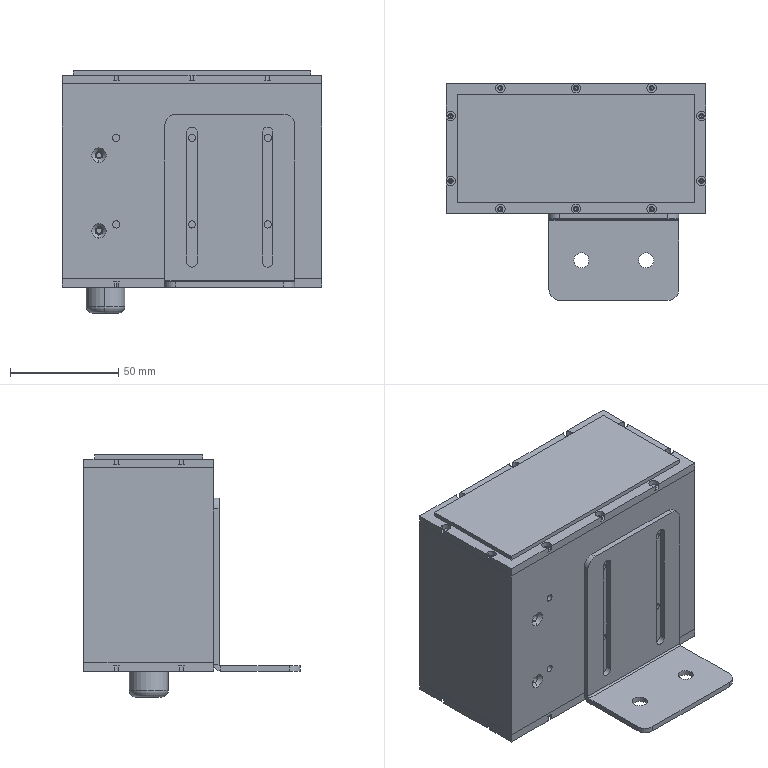Part | SolidWorks | 13 solids | 366 faces | box 120 x 100 x 112 mm | volume 221397 mm3 | cylinder 208 | plane 106 | cone 48 | torus 4 | commonest cylinder face diameters 4.4 x42 1.6 x40 2.4 x40 3.3 x24 2.5 x16 3.4 x8